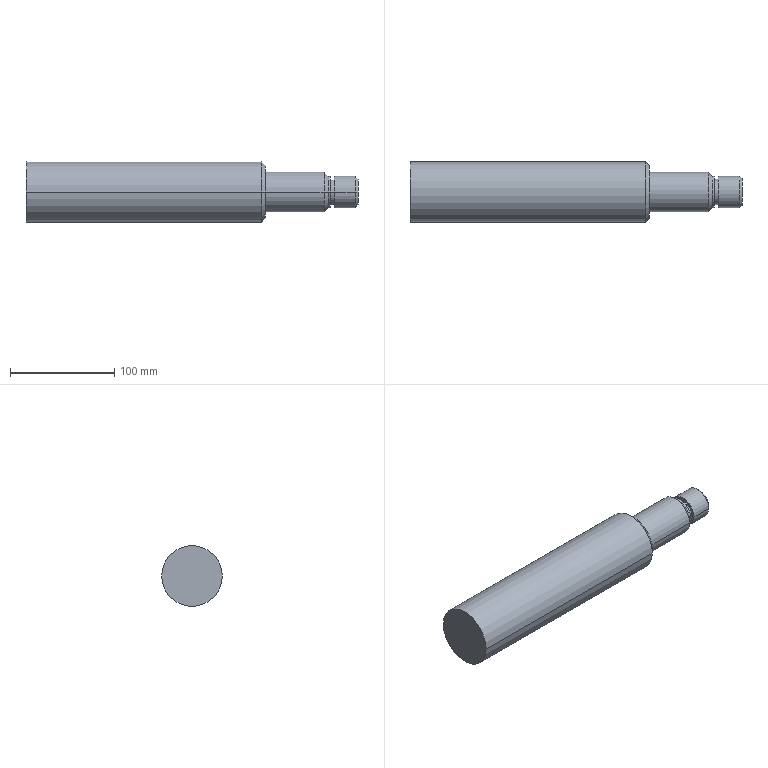Part | SolidWorks | features Revolution 1 | 1 solid | 21 faces | box 317.85 x 58 x 58 mm | volume 690126 mm3 | cylinder 10 | cone 6 | plane 5 | commonest cylinder face diameters 30 x4 24 x2 38 x2 58 x2
STEP:
#1=CARTESIAN_POINT('',(830.873,12.5,0.));
#2=VERTEX_POINT('',#1);
#3=CARTESIAN_POINT('',(830.873,-12.5,0.));
#4=VERTEX_POINT('',#3);
#5=CARTESIAN_POINT('',(830.873,0.,0.));
#6=DIRECTION('',(1.,0.,0.));
#7=DIRECTION('',(0.,1.,0.));
#8=AXIS2_PLACEMENT_3D('',#5,#6,#7);
#9=CIRCLE('',#8,12.5);
#10=EDGE_CURVE('',#2,#4,#9,.T.);
#11=ORIENTED_EDGE('',*,*,#10,.F.);
#12=CARTESIAN_POINT('',(828.373,15.,0.));
#13=VERTEX_POINT('',#12);
#14=CARTESIAN_POINT('',(830.873,12.5,0.));
#15=DIRECTION('',(-0.7071,0.7071,0.));
#16=VECTOR('',#15,1000.);
#17=LINE('',#14,#16);
#18=EDGE_CURVE('',#2,#13,#17,.T.);
#19=ORIENTED_EDGE('',*,*,#18,.T.);
#20=CARTESIAN_POINT('',(828.373,-15.,0.));
#21=VERTEX_POINT('',#20);
#22=CARTESIAN_POINT('',(828.373,0.,0.));
#23=DIRECTION('',(1.,0.,0.));
#24=DIRECTION('',(0.,1.,0.));
#25=AXIS2_PLACEMENT_3D('',#22,#23,#24);
#26=CIRCLE('',#25,15.);
#27=EDGE_CURVE('',#13,#21,#26,.T.);
#28=ORIENTED_EDGE('',*,*,#27,.T.);
#29=CARTESIAN_POINT('',(830.873,-12.5,0.));
#30=DIRECTION('',(-0.7071,-0.7071,0.));
#31=VECTOR('',#30,1000.);
#32=LINE('',#29,#31);
#33=EDGE_CURVE('',#4,#21,#32,.T.);
#34=ORIENTED_EDGE('',*,*,#33,.F.);
#35=EDGE_LOOP('',(#11,#19,#28,#34));
#36=FACE_OUTER_BOUND('',#35,.T.);
#37=CARTESIAN_POINT('',(830.873,0.,0.));
#38=DIRECTION('',(-1.,0.,0.));
#39=DIRECTION('',(0.,-1.,0.));
#40=AXIS2_PLACEMENT_3D('',#37,#38,#39);
#41=CONICAL_SURFACE('',#40,12.5,0.7854);
#42=ADVANCED_FACE('',(#36),#41,.T.);
#43=CARTESIAN_POINT('',(808.373,15.,0.));
#44=VERTEX_POINT('',#43);
#45=CARTESIAN_POINT('',(808.373,-15.,0.));
#46=VERTEX_POINT('',#45);
#47=CARTESIAN_POINT('',(808.373,0.,0.));
#48=DIRECTION('',(1.,0.,0.));
#49=DIRECTION('',(0.,1.,0.));
#50=AXIS2_PLACEMENT_3D('',#47,#48,#49);
#51=CIRCLE('',#50,15.);
#52=EDGE_CURVE('',#44,#46,#51,.T.);
#53=ORIENTED_EDGE('',*,*,#52,.T.);
#54=CARTESIAN_POINT('',(838.373,-15.,0.));
#55=DIRECTION('',(1.,0.,0.));
#56=VECTOR('',#55,1000.);
#57=LINE('',#54,#56);
#58=EDGE_CURVE('',#46,#21,#57,.T.);
#59=ORIENTED_EDGE('',*,*,#58,.T.);
#60=ORIENTED_EDGE('',*,*,#27,.F.);
#61=CARTESIAN_POINT('',(838.373,15.,0.));
#62=DIRECTION('',(1.,0.,0.));
#63=VECTOR('',#62,1000.);
#64=LINE('',#61,#63);
#65=EDGE_CURVE('',#44,#13,#64,.T.);
#66=ORIENTED_EDGE('',*,*,#65,.F.);
#67=EDGE_LOOP('',(#53,#59,#60,#66));
#68=FACE_OUTER_BOUND('',#67,.T.);
#69=CARTESIAN_POINT('',(838.373,0.,0.));
#70=DIRECTION('',(1.,0.,0.));
#71=DIRECTION('',(0.,1.,0.));
#72=AXIS2_PLACEMENT_3D('',#69,#70,#71);
#73=CYLINDRICAL_SURFACE('',#72,15.);
#74=ADVANCED_FACE('',(#68),#73,.T.);
#75=CARTESIAN_POINT('',(804.373,12.,0.));
#76=VERTEX_POINT('',#75);
#77=CARTESIAN_POINT('',(804.373,-12.,0.));
#78=VERTEX_POINT('',#77);
#79=CARTESIAN_POINT('',(804.373,0.,0.));
#80=DIRECTION('',(1.,0.,0.));
#81=DIRECTION('',(0.,1.,0.));
#82=AXIS2_PLACEMENT_3D('',#79,#80,#81);
#83=CIRCLE('',#82,12.);
#84=EDGE_CURVE('',#76,#78,#83,.T.);
#85=ORIENTED_EDGE('',*,*,#84,.T.);
#86=CARTESIAN_POINT('',(808.373,-12.,0.));
#87=VERTEX_POINT('',#86);
#88=CARTESIAN_POINT('',(838.373,-12.,0.));
#89=DIRECTION('',(1.,0.,0.));
#90=VECTOR('',#89,1000.);
#91=LINE('',#88,#90);
#92=EDGE_CURVE('',#78,#87,#91,.T.);
#93=ORIENTED_EDGE('',*,*,#92,.T.);
#94=CARTESIAN_POINT('',(808.373,12.,0.));
#95=VERTEX_POINT('',#94);
#96=CARTESIAN_POINT('',(808.373,0.,0.));
#97=DIRECTION('',(1.,0.,0.));
#98=DIRECTION('',(0.,1.,0.));
#99=AXIS2_PLACEMENT_3D('',#96,#97,#98);
#100=CIRCLE('',#99,12.);
#101=EDGE_CURVE('',#95,#87,#100,.T.);
#102=ORIENTED_EDGE('',*,*,#101,.F.);
#103=CARTESIAN_POINT('',(838.373,12.,0.));
#104=DIRECTION('',(1.,0.,0.));
#105=VECTOR('',#104,1000.);
#106=LINE('',#103,#105);
#107=EDGE_CURVE('',#76,#95,#106,.T.);
#108=ORIENTED_EDGE('',*,*,#107,.F.);
#109=EDGE_LOOP('',(#85,#93,#102,#108));
#110=FACE_OUTER_BOUND('',#109,.T.);
#111=CARTESIAN_POINT('',(838.373,0.,0.));
#112=DIRECTION('',(1.,0.,0.));
#113=DIRECTION('',(0.,1.,0.));
#114=AXIS2_PLACEMENT_3D('',#111,#112,#113);
#115=CYLINDRICAL_SURFACE('',#114,12.);
#116=ADVANCED_FACE('',(#110),#115,.T.);
#117=CARTESIAN_POINT('',(802.373,15.,0.));
#118=VERTEX_POINT('',#117);
#119=CARTESIAN_POINT('',(802.373,-15.,0.));
#120=VERTEX_POINT('',#119);
#121=CARTESIAN_POINT('',(802.373,0.,0.));
#122=DIRECTION('',(1.,0.,0.));
#123=DIRECTION('',(0.,1.,0.));
#124=AXIS2_PLACEMENT_3D('',#121,#122,#123);
#125=CIRCLE('',#124,15.);
#126=EDGE_CURVE('',#118,#120,#125,.T.);
#127=ORIENTED_EDGE('',*,*,#126,.T.);
#128=CARTESIAN_POINT('',(804.373,-15.,0.));
#129=VERTEX_POINT('',#128);
#130=CARTESIAN_POINT('',(838.373,-15.,0.));
#131=DIRECTION('',(1.,0.,0.));
#132=VECTOR('',#131,1000.);
#133=LINE('',#130,#132);
#134=EDGE_CURVE('',#120,#129,#133,.T.);
#135=ORIENTED_EDGE('',*,*,#134,.T.);
#136=CARTESIAN_POINT('',(804.373,15.,0.));
#137=VERTEX_POINT('',#136);
#138=CARTESIAN_POINT('',(804.373,0.,0.));
#139=DIRECTION('',(1.,0.,0.));
#140=DIRECTION('',(0.,1.,0.));
#141=AXIS2_PLACEMENT_3D('',#138,#139,#140);
#142=CIRCLE('',#141,15.);
#143=EDGE_CURVE('',#137,#129,#142,.T.);
#144=ORIENTED_EDGE('',*,*,#143,.F.);
#145=CARTESIAN_POINT('',(838.373,15.,0.));
#146=DIRECTION('',(1.,0.,0.));
#147=VECTOR('',#146,1000.);
#148=LINE('',#145,#147);
#149=EDGE_CURVE('',#118,#137,#148,.T.);
#150=ORIENTED_EDGE('',*,*,#149,.F.);
#151=EDGE_LOOP('',(#127,#135,#144,#150));
#152=FACE_OUTER_BOUND('',#151,.T.);
#153=CARTESIAN_POINT('',(838.373,0.,0.));
#154=DIRECTION('',(1.,0.,0.));
#155=DIRECTION('',(0.,1.,0.));
#156=AXIS2_PLACEMENT_3D('',#153,#154,#155);
#157=CYLINDRICAL_SURFACE('',#156,15.);
#158=ADVANCED_FACE('',(#152),#157,.T.);
#159=ORIENTED_EDGE('',*,*,#126,.F.);
#160=CARTESIAN_POINT('',(798.373,19.,0.));
#161=VERTEX_POINT('',#160);
#162=CARTESIAN_POINT('',(802.373,15.,0.));
#163=DIRECTION('',(-0.7071,0.7071,0.));
#164=VECTOR('',#163,1000.);
#165=LINE('',#162,#164);
#166=EDGE_CURVE('',#118,#161,#165,.T.);
#167=ORIENTED_EDGE('',*,*,#166,.T.);
#168=CARTESIAN_POINT('',(798.373,-19.,0.));
#169=VERTEX_POINT('',#168);
#170=CARTESIAN_POINT('',(798.373,0.,0.));
#171=DIRECTION('',(1.,0.,0.));
#172=DIRECTION('',(0.,1.,0.));
#173=AXIS2_PLACEMENT_3D('',#170,#171,#172);
#174=CIRCLE('',#173,19.);
#175=EDGE_CURVE('',#161,#169,#174,.T.);
#176=ORIENTED_EDGE('',*,*,#175,.T.);
#177=CARTESIAN_POINT('',(802.373,-15.,0.));
#178=DIRECTION('',(-0.7071,-0.7071,0.));
#179=VECTOR('',#178,1000.);
#180=LINE('',#177,#179);
#181=EDGE_CURVE('',#120,#169,#180,.T.);
#182=ORIENTED_EDGE('',*,*,#181,.F.);
#183=EDGE_LOOP('',(#159,#167,#176,#182));
#184=FACE_OUTER_BOUND('',#183,.T.);
#185=CARTESIAN_POINT('',(802.373,0.,0.));
#186=DIRECTION('',(-1.,0.,0.));
#187=DIRECTION('',(0.,-1.,0.));
#188=AXIS2_PLACEMENT_3D('',#185,#186,#187);
#189=CONICAL_SURFACE('',#188,15.,0.7854);
#190=ADVANCED_FACE('',(#184),#189,.T.);
#191=CARTESIAN_POINT('',(742.073,19.,0.));
#192=VERTEX_POINT('',#191);
#193=CARTESIAN_POINT('',(742.073,-19.,0.));
#194=VERTEX_POINT('',#193);
#195=CARTESIAN_POINT('',(742.073,0.,0.));
#196=DIRECTION('',(1.,0.,0.));
#197=DIRECTION('',(0.,1.,0.));
#198=AXIS2_PLACEMENT_3D('',#195,#196,#197);
#199=CIRCLE('',#198,19.);
#200=EDGE_CURVE('',#192,#194,#199,.T.);
#201=ORIENTED_EDGE('',*,*,#200,.T.);
#202=CARTESIAN_POINT('',(838.373,-19.,0.));
#203=DIRECTION('',(1.,0.,0.));
#204=VECTOR('',#203,1000.);
#205=LINE('',#202,#204);
#206=EDGE_CURVE('',#194,#169,#205,.T.);
#207=ORIENTED_EDGE('',*,*,#206,.T.);
#208=ORIENTED_EDGE('',*,*,#175,.F.);
#209=CARTESIAN_POINT('',(838.373,19.,0.));
#210=DIRECTION('',(1.,0.,0.));
#211=VECTOR('',#210,1000.);
#212=LINE('',#209,#211);
#213=EDGE_CURVE('',#192,#161,#212,.T.);
#214=ORIENTED_EDGE('',*,*,#213,.F.);
#215=EDGE_LOOP('',(#201,#207,#208,#214));
#216=FACE_OUTER_BOUND('',#215,.T.);
#217=CARTESIAN_POINT('',(838.373,0.,0.));
#218=DIRECTION('',(1.,0.,0.));
#219=DIRECTION('',(0.,1.,0.));
#220=AXIS2_PLACEMENT_3D('',#217,#218,#219);
#221=CYLINDRICAL_SURFACE('',#220,19.);
#222=ADVANCED_FACE('',(#216),#221,.T.);
#223=CARTESIAN_POINT('',(742.073,25.,0.));
#224=VERTEX_POINT('',#223);
#225=CARTESIAN_POINT('',(742.073,-25.,0.));
#226=VERTEX_POINT('',#225);
#227=CARTESIAN_POINT('',(742.073,0.,0.));
#228=DIRECTION('',(1.,0.,0.));
#229=DIRECTION('',(0.,1.,0.));
#230=AXIS2_PLACEMENT_3D('',#227,#228,#229);
#231=CIRCLE('',#230,25.);
#232=EDGE_CURVE('',#224,#226,#231,.T.);
#233=ORIENTED_EDGE('',*,*,#232,.F.);
#234=CARTESIAN_POINT('',(738.073,29.,0.));
#235=VERTEX_POINT('',#234);
#236=CARTESIAN_POINT('',(742.073,25.,0.));
#237=DIRECTION('',(-0.7071,0.7071,0.));
#238=VECTOR('',#237,1000.);
#239=LINE('',#236,#238);
#240=EDGE_CURVE('',#224,#235,#239,.T.);
#241=ORIENTED_EDGE('',*,*,#240,.T.);
#242=CARTESIAN_POINT('',(738.073,-29.,0.));
#243=VERTEX_POINT('',#242);
#244=CARTESIAN_POINT('',(738.073,0.,0.));
#245=DIRECTION('',(1.,0.,0.));
#246=DIRECTION('',(0.,1.,0.));
#247=AXIS2_PLACEMENT_3D('',#244,#245,#246);
#248=CIRCLE('',#247,29.);
#249=EDGE_CURVE('',#235,#243,#248,.T.);
#250=ORIENTED_EDGE('',*,*,#249,.T.);
#251=CARTESIAN_POINT('',(742.073,-25.,0.));
#252=DIRECTION('',(-0.7071,-0.7071,0.));
#253=VECTOR('',#252,1000.);
#254=LINE('',#251,#253);
#255=EDGE_CURVE('',#226,#243,#254,.T.);
#256=ORIENTED_EDGE('',*,*,#255,.F.);
#257=EDGE_LOOP('',(#233,#241,#250,#256));
#258=FACE_OUTER_BOUND('',#257,.T.);
#259=CARTESIAN_POINT('',(742.073,0.,0.));
#260=DIRECTION('',(-1.,0.,0.));
#261=DIRECTION('',(0.,-1.,0.));
#262=AXIS2_PLACEMENT_3D('',#259,#260,#261);
#263=CONICAL_SURFACE('',#262,25.,0.7854);
#264=ADVANCED_FACE('',(#258),#263,.T.);
#265=CARTESIAN_POINT('',(513.023,29.,0.));
#266=VERTEX_POINT('',#265);
#267=CARTESIAN_POINT('',(513.023,-29.,0.));
#268=VERTEX_POINT('',#267);
#269=CARTESIAN_POINT('',(513.023,0.,0.));
#270=DIRECTION('',(1.,0.,0.));
#271=DIRECTION('',(0.,1.,0.));
#272=AXIS2_PLACEMENT_3D('',#269,#270,#271);
#273=CIRCLE('',#272,29.);
#274=EDGE_CURVE('',#266,#268,#273,.T.);
#275=ORIENTED_EDGE('',*,*,#274,.T.);
#276=CARTESIAN_POINT('',(838.373,-29.,0.));
#277=DIRECTION('',(1.,0.,0.));
#278=VECTOR('',#277,1000.);
#279=LINE('',#276,#278);
#280=EDGE_CURVE('',#268,#243,#279,.T.);
#281=ORIENTED_EDGE('',*,*,#280,.T.);
#282=ORIENTED_EDGE('',*,*,#249,.F.);
#283=CARTESIAN_POINT('',(838.373,29.,0.));
#284=DIRECTION('',(1.,0.,0.));
#285=VECTOR('',#284,1000.);
#286=LINE('',#283,#285);
#287=EDGE_CURVE('',#266,#235,#286,.T.);
#288=ORIENTED_EDGE('',*,*,#287,.F.);
#289=EDGE_LOOP('',(#275,#281,#282,#288));
#290=FACE_OUTER_BOUND('',#289,.T.);
#291=CARTESIAN_POINT('',(838.373,0.,0.));
#292=DIRECTION('',(1.,0.,0.));
#293=DIRECTION('',(0.,1.,0.));
#294=AXIS2_PLACEMENT_3D('',#291,#292,#293);
#295=CYLINDRICAL_SURFACE('',#294,29.);
#296=ADVANCED_FACE('',(#290),#295,.T.);
#297=ORIENTED_EDGE('',*,*,#274,.F.);
#298=CARTESIAN_POINT('',(513.023,0.,0.));
#299=DIRECTION('',(1.,0.,0.));
#300=DIRECTION('',(0.,1.,0.));
#301=AXIS2_PLACEMENT_3D('',#298,#299,#300);
#302=CIRCLE('',#301,29.);
#303=EDGE_CURVE('',#268,#266,#302,.T.);
#304=ORIENTED_EDGE('',*,*,#303,.F.);
#305=EDGE_LOOP('',(#297,#304));
#306=FACE_OUTER_BOUND('',#305,.T.);
#307=CARTESIAN_POINT('',(513.023,29.,0.));
#308=DIRECTION('',(-1.,0.,0.));
#309=DIRECTION('',(0.,-1.,0.));
#310=AXIS2_PLACEMENT_3D('',#307,#308,#309);
#311=PLANE('',#310);
#312=ADVANCED_FACE('',(#306),#311,.T.);
#313=ORIENTED_EDGE('',*,*,#280,.F.);
#314=ORIENTED_EDGE('',*,*,#303,.T.);
#315=ORIENTED_EDGE('',*,*,#287,.T.);
#316=CARTESIAN_POINT('',(738.073,0.,0.));
#317=DIRECTION('',(1.,0.,0.));
#318=DIRECTION('',(0.,1.,0.));
#319=AXIS2_PLACEMENT_3D('',#316,#317,#318);
#320=CIRCLE('',#319,29.);
#321=EDGE_CURVE('',#243,#235,#320,.T.);
#322=ORIENTED_EDGE('',*,*,#321,.F.);
#323=EDGE_LOOP('',(#313,#314,#315,#322));
#324=FACE_OUTER_BOUND('',#323,.T.);
#325=CARTESIAN_POINT('',(838.373,0.,0.));
#326=DIRECTION('',(1.,0.,0.));
#327=DIRECTION('',(0.,1.,0.));
#328=AXIS2_PLACEMENT_3D('',#325,#326,#327);
#329=CYLINDRICAL_SURFACE('',#328,29.);
#330=ADVANCED_FACE('',(#324),#329,.T.);
#331=ORIENTED_EDGE('',*,*,#240,.F.);
#332=CARTESIAN_POINT('',(742.073,0.,0.));
#333=DIRECTION('',(1.,0.,0.));
#334=DIRECTION('',(0.,1.,0.));
#335=AXIS2_PLACEMENT_3D('',#332,#333,#334);
#336=CIRCLE('',#335,25.);
#337=EDGE_CURVE('',#226,#224,#336,.T.);
#338=ORIENTED_EDGE('',*,*,#337,.F.);
#339=ORIENTED_EDGE('',*,*,#255,.T.);
#340=ORIENTED_EDGE('',*,*,#321,.T.);
#341=EDGE_LOOP('',(#331,#338,#339,#340));
#342=FACE_OUTER_BOUND('',#341,.T.);
#343=CARTESIAN_POINT('',(742.073,0.,0.));
#344=DIRECTION('',(-1.,0.,0.));
#345=DIRECTION('',(0.,-1.,0.));
#346=AXIS2_PLACEMENT_3D('',#343,#344,#345);
#347=CONICAL_SURFACE('',#346,25.,0.7854);
#348=ADVANCED_FACE('',(#342),#347,.T.);
#349=ORIENTED_EDGE('',*,*,#337,.T.);
#350=ORIENTED_EDGE('',*,*,#232,.T.);
#351=EDGE_LOOP('',(#349,#350));
#352=FACE_OUTER_BOUND('',#351,.T.);
#353=ORIENTED_EDGE('',*,*,#200,.F.);
#354=CARTESIAN_POINT('',(742.073,0.,0.));
#355=DIRECTION('',(1.,0.,0.));
#356=DIRECTION('',(0.,1.,0.));
#357=AXIS2_PLACEMENT_3D('',#354,#355,#356);
#358=CIRCLE('',#357,19.);
#359=EDGE_CURVE('',#194,#192,#358,.T.);
#360=ORIENTED_EDGE('',*,*,#359,.F.);
#361=EDGE_LOOP('',(#353,#360));
#362=FACE_BOUND('',#361,.T.);
#363=CARTESIAN_POINT('',(742.073,25.,0.));
#364=DIRECTION('',(1.,0.,0.));
#365=DIRECTION('',(0.,1.,0.));
#366=AXIS2_PLACEMENT_3D('',#363,#364,#365);
#367=PLANE('',#366);
#368=ADVANCED_FACE('',(#352,#362),#367,.T.);
#369=ORIENTED_EDGE('',*,*,#206,.F.);
#370=ORIENTED_EDGE('',*,*,#359,.T.);
#371=ORIENTED_EDGE('',*,*,#213,.T.);
#372=CARTESIAN_POINT('',(798.373,0.,0.));
#373=DIRECTION('',(1.,0.,0.));
#374=DIRECTION('',(0.,1.,0.));
#375=AXIS2_PLACEMENT_3D('',#372,#373,#374);
#376=CIRCLE('',#375,19.);
#377=EDGE_CURVE('',#169,#161,#376,.T.);
#378=ORIENTED_EDGE('',*,*,#377,.F.);
#379=EDGE_LOOP('',(#369,#370,#371,#378));
#380=FACE_OUTER_BOUND('',#379,.T.);
#381=CARTESIAN_POINT('',(838.373,0.,0.));
#382=DIRECTION('',(1.,0.,0.));
#383=DIRECTION('',(0.,1.,0.));
#384=AXIS2_PLACEMENT_3D('',#381,#382,#383);
#385=CYLINDRICAL_SURFACE('',#384,19.);
#386=ADVANCED_FACE('',(#380),#385,.T.);
#387=ORIENTED_EDGE('',*,*,#166,.F.);
#388=CARTESIAN_POINT('',(802.373,0.,0.));
#389=DIRECTION('',(1.,0.,0.));
#390=DIRECTION('',(0.,1.,0.));
#391=AXIS2_PLACEMENT_3D('',#388,#389,#390);
#392=CIRCLE('',#391,15.);
#393=EDGE_CURVE('',#120,#118,#392,.T.);
#394=ORIENTED_EDGE('',*,*,#393,.F.);
#395=ORIENTED_EDGE('',*,*,#181,.T.);
#396=ORIENTED_EDGE('',*,*,#377,.T.);
#397=EDGE_LOOP('',(#387,#394,#395,#396));
#398=FACE_OUTER_BOUND('',#397,.T.);
#399=CARTESIAN_POINT('',(802.373,0.,0.));
#400=DIRECTION('',(-1.,0.,0.));
#401=DIRECTION('',(0.,-1.,0.));
#402=AXIS2_PLACEMENT_3D('',#399,#400,#401);
#403=CONICAL_SURFACE('',#402,15.,0.7854);
#404=ADVANCED_FACE('',(#398),#403,.T.);
#405=ORIENTED_EDGE('',*,*,#134,.F.);
#406=ORIENTED_EDGE('',*,*,#393,.T.);
#407=ORIENTED_EDGE('',*,*,#149,.T.);
#408=CARTESIAN_POINT('',(804.373,0.,0.));
#409=DIRECTION('',(1.,0.,0.));
#410=DIRECTION('',(0.,1.,0.));
#411=AXIS2_PLACEMENT_3D('',#408,#409,#410);
#412=CIRCLE('',#411,15.);
#413=EDGE_CURVE('',#129,#137,#412,.T.);
#414=ORIENTED_EDGE('',*,*,#413,.F.);
#415=EDGE_LOOP('',(#405,#406,#407,#414));
#416=FACE_OUTER_BOUND('',#415,.T.);
#417=CARTESIAN_POINT('',(838.373,0.,0.));
#418=DIRECTION('',(1.,0.,0.));
#419=DIRECTION('',(0.,1.,0.));
#420=AXIS2_PLACEMENT_3D('',#417,#418,#419);
#421=CYLINDRICAL_SURFACE('',#420,15.);
#422=ADVANCED_FACE('',(#416),#421,.T.);
#423=ORIENTED_EDGE('',*,*,#143,.T.);
#424=ORIENTED_EDGE('',*,*,#413,.T.);
#425=EDGE_LOOP('',(#423,#424));
#426=FACE_OUTER_BOUND('',#425,.T.);
#427=ORIENTED_EDGE('',*,*,#84,.F.);
#428=CARTESIAN_POINT('',(804.373,0.,0.));
#429=DIRECTION('',(1.,0.,0.));
#430=DIRECTION('',(0.,1.,0.));
#431=AXIS2_PLACEMENT_3D('',#428,#429,#430);
#432=CIRCLE('',#431,12.);
#433=EDGE_CURVE('',#78,#76,#432,.T.);
#434=ORIENTED_EDGE('',*,*,#433,.F.);
#435=EDGE_LOOP('',(#427,#434));
#436=FACE_BOUND('',#435,.T.);
#437=CARTESIAN_POINT('',(804.373,15.,0.));
#438=DIRECTION('',(1.,0.,0.));
#439=DIRECTION('',(0.,1.,0.));
#440=AXIS2_PLACEMENT_3D('',#437,#438,#439);
#441=PLANE('',#440);
#442=ADVANCED_FACE('',(#426,#436),#441,.T.);
#443=ORIENTED_EDGE('',*,*,#92,.F.);
#444=ORIENTED_EDGE('',*,*,#433,.T.);
#445=ORIENTED_EDGE('',*,*,#107,.T.);
#446=CARTESIAN_POINT('',(808.373,0.,0.));
#447=DIRECTION('',(1.,0.,0.));
#448=DIRECTION('',(0.,1.,0.));
#449=AXIS2_PLACEMENT_3D('',#446,#447,#448);
#450=CIRCLE('',#449,12.);
#451=EDGE_CURVE('',#87,#95,#450,.T.);
#452=ORIENTED_EDGE('',*,*,#451,.F.);
#453=EDGE_LOOP('',(#443,#444,#445,#452));
#454=FACE_OUTER_BOUND('',#453,.T.);
#455=CARTESIAN_POINT('',(838.373,0.,0.));
#456=DIRECTION('',(1.,0.,0.));
#457=DIRECTION('',(0.,1.,0.));
#458=AXIS2_PLACEMENT_3D('',#455,#456,#457);
#459=CYLINDRICAL_SURFACE('',#458,12.);
#460=ADVANCED_FACE('',(#454),#459,.T.);
#461=ORIENTED_EDGE('',*,*,#101,.T.);
#462=ORIENTED_EDGE('',*,*,#451,.T.);
#463=EDGE_LOOP('',(#461,#462));
#464=FACE_BOUND('',#463,.T.);
#465=ORIENTED_EDGE('',*,*,#52,.F.);
#466=CARTESIAN_POINT('',(808.373,0.,0.));
#467=DIRECTION('',(1.,0.,0.));
#468=DIRECTION('',(0.,1.,0.));
#469=AXIS2_PLACEMENT_3D('',#466,#467,#468);
#470=CIRCLE('',#469,15.);
#471=EDGE_CURVE('',#46,#44,#470,.T.);
#472=ORIENTED_EDGE('',*,*,#471,.F.);
#473=EDGE_LOOP('',(#465,#472));
#474=FACE_OUTER_BOUND('',#473,.T.);
#475=CARTESIAN_POINT('',(808.373,15.,0.));
#476=DIRECTION('',(-1.,0.,0.));
#477=DIRECTION('',(0.,-1.,0.));
#478=AXIS2_PLACEMENT_3D('',#475,#476,#477);
#479=PLANE('',#478);
#480=ADVANCED_FACE('',(#464,#474),#479,.T.);
#481=ORIENTED_EDGE('',*,*,#58,.F.);
#482=ORIENTED_EDGE('',*,*,#471,.T.);
#483=ORIENTED_EDGE('',*,*,#65,.T.);
#484=CARTESIAN_POINT('',(828.373,0.,0.));
#485=DIRECTION('',(1.,0.,0.));
#486=DIRECTION('',(0.,1.,0.));
#487=AXIS2_PLACEMENT_3D('',#484,#485,#486);
#488=CIRCLE('',#487,15.);
#489=EDGE_CURVE('',#21,#13,#488,.T.);
#490=ORIENTED_EDGE('',*,*,#489,.F.);
#491=EDGE_LOOP('',(#481,#482,#483,#490));
#492=FACE_OUTER_BOUND('',#491,.T.);
#493=CARTESIAN_POINT('',(838.373,0.,0.));
#494=DIRECTION('',(1.,0.,0.));
#495=DIRECTION('',(0.,1.,0.));
#496=AXIS2_PLACEMENT_3D('',#493,#494,#495);
#497=CYLINDRICAL_SURFACE('',#496,15.);
#498=ADVANCED_FACE('',(#492),#497,.T.);
#499=ORIENTED_EDGE('',*,*,#18,.F.);
#500=CARTESIAN_POINT('',(830.873,0.,0.));
#501=DIRECTION('',(1.,0.,0.));
#502=DIRECTION('',(0.,1.,0.));
#503=AXIS2_PLACEMENT_3D('',#500,#501,#502);
#504=CIRCLE('',#503,12.5);
#505=EDGE_CURVE('',#4,#2,#504,.T.);
#506=ORIENTED_EDGE('',*,*,#505,.F.);
#507=ORIENTED_EDGE('',*,*,#33,.T.);
#508=ORIENTED_EDGE('',*,*,#489,.T.);
#509=EDGE_LOOP('',(#499,#506,#507,#508));
#510=FACE_OUTER_BOUND('',#509,.T.);
#511=CARTESIAN_POINT('',(830.873,0.,0.));
#512=DIRECTION('',(-1.,0.,0.));
#513=DIRECTION('',(0.,-1.,0.));
#514=AXIS2_PLACEMENT_3D('',#511,#512,#513);
#515=CONICAL_SURFACE('',#514,12.5,0.7854);
#516=ADVANCED_FACE('',(#510),#515,.T.);
#517=ORIENTED_EDGE('',*,*,#505,.T.);
#518=ORIENTED_EDGE('',*,*,#10,.T.);
#519=EDGE_LOOP('',(#517,#518));
#520=FACE_OUTER_BOUND('',#519,.T.);
#521=CARTESIAN_POINT('',(830.873,12.5,0.));
#522=DIRECTION('',(1.,0.,0.));
#523=DIRECTION('',(0.,1.,0.));
#524=AXIS2_PLACEMENT_3D('',#521,#522,#523);
#525=PLANE('',#524);
#526=ADVANCED_FACE('',(#520),#525,.T.);
#527=CLOSED_SHELL('',(#42,#74,#116,#158,#190,#222,#264,#296,#312,#330,#348,#368,#386,#404,#422,#442,#460,#480,#498,#516,#526));
#528=MANIFOLD_SOLID_BREP('',#527);
#529=CARTESIAN_POINT('',(0.,0.,0.));
#530=DIRECTION('',(0.,0.,1.));
#531=DIRECTION('',(1.,0.,0.));
#532=AXIS2_PLACEMENT_3D('',#529,#530,#531);
#533=(LENGTH_UNIT()NAMED_UNIT(*)SI_UNIT(.MILLI.,.METRE.));
#534=UNCERTAINTY_MEASURE_WITH_UNIT(LENGTH_MEASURE(0.00001),#533,'','');
#535=(NAMED_UNIT(*)PLANE_ANGLE_UNIT()SI_UNIT($,.RADIAN.));
#536=(NAMED_UNIT(*)SI_UNIT($,.STERADIAN.)SOLID_ANGLE_UNIT());
#537=(GEOMETRIC_REPRESENTATION_CONTEXT(3)GLOBAL_UNCERTAINTY_ASSIGNED_CONTEXT((#534))GLOBAL_UNIT_ASSIGNED_CONTEXT((#533,#535,#536))REPRESENTATION_CONTEXT('',''));
#538=ADVANCED_BREP_SHAPE_REPRESENTATION('',(#528,#532),#537);